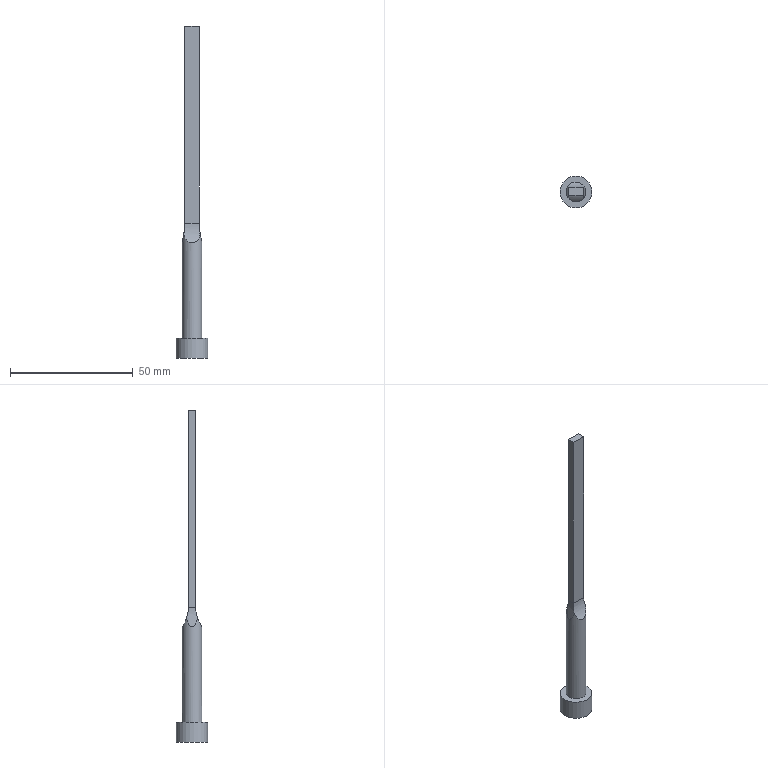Part | STEP file | DDZ8.00_id210_x_t | 1 solid | 13 faces | box 13 x 13 x 135.432 mm | volume 4709 mm3 | plane 7 | cylinder 6 | commonest cylinder face diameters 28.1 x2 65 x2 8 x1 13 x1
STEP:
#1=CARTESIAN_POINT('',(-3.313,-55.759,-85.002));
#2=VERTEX_POINT('',#1);
#3=CARTESIAN_POINT('',(-3.313,-60.241,-85.002));
#4=VERTEX_POINT('',#3);
#5=CARTESIAN_POINT('',(-3.313,-55.759,-85.002));
#6=CARTESIAN_POINT('',(-3.415,-55.909,-85.727));
#7=CARTESIAN_POINT('',(-3.54,-56.104,-86.436));
#8=CARTESIAN_POINT('',(-3.746,-56.586,-87.431));
#9=CARTESIAN_POINT('',(-3.817,-56.776,-87.747));
#10=CARTESIAN_POINT('',(-3.945,-57.286,-88.284));
#11=CARTESIAN_POINT('',(-4.,-57.628,-88.501));
#12=CARTESIAN_POINT('',(-4.,-58.379,-88.499));
#13=CARTESIAN_POINT('',(-3.943,-58.723,-88.276));
#14=CARTESIAN_POINT('',(-3.816,-59.229,-87.74));
#15=CARTESIAN_POINT('',(-3.743,-59.42,-87.42));
#16=CARTESIAN_POINT('',(-3.539,-59.896,-86.433));
#17=CARTESIAN_POINT('',(-3.415,-60.091,-85.726));
#18=CARTESIAN_POINT('',(-3.313,-60.241,-85.002));
#19=B_SPLINE_CURVE_WITH_KNOTS('',3,(#5,#6,#7,#8,#9,#10,#11,#12,#13,#14,#15,#16,#17,#18),.UNSPECIFIED.,.F.,.F.,(4,2,2,2,2,2,4),(0.,0.25,0.375,0.5,0.625,0.75,1.),.UNSPECIFIED.);
#20=EDGE_CURVE('',#2,#4,#19,.T.);
#21=ORIENTED_EDGE('',*,*,#20,.F.);
#22=CARTESIAN_POINT('',(3.313,-55.759,-85.002));
#23=VERTEX_POINT('',#22);
#24=CARTESIAN_POINT('',(3.313,-55.759,-85.002));
#25=CARTESIAN_POINT('',(3.117,-55.468,-85.861));
#26=CARTESIAN_POINT('',(2.822,-55.093,-86.676));
#27=CARTESIAN_POINT('',(1.767,-54.354,-88.002));
#28=CARTESIAN_POINT('',(0.9205,-54.,-88.501));
#29=CARTESIAN_POINT('',(-0.9239,-54.,-88.499));
#30=CARTESIAN_POINT('',(-1.772,-54.357,-87.997));
#31=CARTESIAN_POINT('',(-2.822,-55.094,-86.673));
#32=CARTESIAN_POINT('',(-3.117,-55.469,-85.861));
#33=CARTESIAN_POINT('',(-3.313,-55.759,-85.002));
#34=B_SPLINE_CURVE_WITH_KNOTS('',3,(#24,#25,#26,#27,#28,#29,#30,#31,#32,#33),.UNSPECIFIED.,.F.,.F.,(4,2,2,2,4),(0.,0.25,0.5,0.75,1.),.UNSPECIFIED.);
#35=EDGE_CURVE('',#23,#2,#34,.T.);
#36=ORIENTED_EDGE('',*,*,#35,.F.);
#37=CARTESIAN_POINT('',(3.313,-60.241,-85.002));
#38=VERTEX_POINT('',#37);
#39=CARTESIAN_POINT('',(3.313,-60.241,-85.002));
#40=CARTESIAN_POINT('',(3.415,-60.091,-85.727));
#41=CARTESIAN_POINT('',(3.54,-59.896,-86.436));
#42=CARTESIAN_POINT('',(3.746,-59.414,-87.431));
#43=CARTESIAN_POINT('',(3.817,-59.224,-87.747));
#44=CARTESIAN_POINT('',(3.945,-58.714,-88.284));
#45=CARTESIAN_POINT('',(4.,-58.372,-88.501));
#46=CARTESIAN_POINT('',(4.,-57.621,-88.499));
#47=CARTESIAN_POINT('',(3.943,-57.277,-88.276));
#48=CARTESIAN_POINT('',(3.816,-56.771,-87.74));
#49=CARTESIAN_POINT('',(3.743,-56.58,-87.42));
#50=CARTESIAN_POINT('',(3.539,-56.104,-86.433));
#51=CARTESIAN_POINT('',(3.415,-55.909,-85.726));
#52=CARTESIAN_POINT('',(3.313,-55.759,-85.002));
#53=B_SPLINE_CURVE_WITH_KNOTS('',3,(#39,#40,#41,#42,#43,#44,#45,#46,#47,#48,#49,#50,#51,#52),.UNSPECIFIED.,.F.,.F.,(4,2,2,2,2,2,4),(0.,0.25,0.375,0.5,0.625,0.75,1.),.UNSPECIFIED.);
#54=EDGE_CURVE('',#38,#23,#53,.T.);
#55=ORIENTED_EDGE('',*,*,#54,.F.);
#56=CARTESIAN_POINT('',(-3.313,-60.241,-85.002));
#57=CARTESIAN_POINT('',(-3.117,-60.532,-85.861));
#58=CARTESIAN_POINT('',(-2.822,-60.907,-86.676));
#59=CARTESIAN_POINT('',(-1.767,-61.646,-88.002));
#60=CARTESIAN_POINT('',(-0.9205,-62.,-88.501));
#61=CARTESIAN_POINT('',(0.9239,-62.,-88.499));
#62=CARTESIAN_POINT('',(1.772,-61.643,-87.997));
#63=CARTESIAN_POINT('',(2.822,-60.906,-86.673));
#64=CARTESIAN_POINT('',(3.117,-60.531,-85.861));
#65=CARTESIAN_POINT('',(3.313,-60.241,-85.002));
#66=B_SPLINE_CURVE_WITH_KNOTS('',3,(#56,#57,#58,#59,#60,#61,#62,#63,#64,#65),.UNSPECIFIED.,.F.,.F.,(4,2,2,2,4),(0.,0.25,0.5,0.75,1.),.UNSPECIFIED.);
#67=EDGE_CURVE('',#4,#38,#66,.T.);
#68=ORIENTED_EDGE('',*,*,#67,.F.);
#69=EDGE_LOOP('',(#21,#36,#55,#68));
#70=FACE_BOUND('',#69,.T.);
#71=CARTESIAN_POINT('',(0.,-62.,-127.5));
#72=VERTEX_POINT('',#71);
#73=CARTESIAN_POINT('',(0.,-58.,-127.5));
#74=DIRECTION('',(0.,0.,-1.));
#75=DIRECTION('',(0.,-1.,0.));
#76=AXIS2_PLACEMENT_3D('',#73,#74,#75);
#77=CIRCLE('',#76,4.);
#78=EDGE_CURVE('',#72,#72,#77,.T.);
#79=ORIENTED_EDGE('',*,*,#78,.F.);
#80=EDGE_LOOP('',(#79));
#81=FACE_BOUND('',#80,.T.);
#82=CARTESIAN_POINT('',(0.,-58.,-140.5));
#83=DIRECTION('',(0.,0.,1.));
#84=DIRECTION('',(0.,-1.,0.));
#85=AXIS2_PLACEMENT_3D('',#82,#83,#84);
#86=CYLINDRICAL_SURFACE('',#85,4.);
#87=ADVANCED_FACE('',(#70,#81),#86,.T.);
#88=ORIENTED_EDGE('',*,*,#78,.T.);
#89=EDGE_LOOP('',(#88));
#90=FACE_BOUND('',#89,.T.);
#91=CARTESIAN_POINT('',(0.,-51.5,-127.5));
#92=VERTEX_POINT('',#91);
#93=CARTESIAN_POINT('',(0.,-58.,-127.5));
#94=DIRECTION('',(0.,0.,-1.));
#95=DIRECTION('',(0.,1.,0.));
#96=AXIS2_PLACEMENT_3D('',#93,#94,#95);
#97=CIRCLE('',#96,6.5);
#98=EDGE_CURVE('',#92,#92,#97,.T.);
#99=ORIENTED_EDGE('',*,*,#98,.F.);
#100=EDGE_LOOP('',(#99));
#101=FACE_BOUND('',#100,.T.);
#102=CARTESIAN_POINT('',(0.,-58.,-127.5));
#103=DIRECTION('',(0.,0.,1.));
#104=DIRECTION('',(0.,-1.,0.));
#105=AXIS2_PLACEMENT_3D('',#102,#103,#104);
#106=PLANE('',#105);
#107=ADVANCED_FACE('',(#90,#101),#106,.T.);
#108=ORIENTED_EDGE('',*,*,#98,.T.);
#109=EDGE_LOOP('',(#108));
#110=FACE_BOUND('',#109,.T.);
#111=CARTESIAN_POINT('',(0.,-64.5,-135.5));
#112=VERTEX_POINT('',#111);
#113=CARTESIAN_POINT('',(0.,-58.,-135.5));
#114=DIRECTION('',(0.,0.,1.));
#115=DIRECTION('',(0.,-1.,0.));
#116=AXIS2_PLACEMENT_3D('',#113,#114,#115);
#117=CIRCLE('',#116,6.5);
#118=EDGE_CURVE('',#112,#112,#117,.T.);
#119=ORIENTED_EDGE('',*,*,#118,.T.);
#120=EDGE_LOOP('',(#119));
#121=FACE_BOUND('',#120,.T.);
#122=CARTESIAN_POINT('',(0.,-58.,-135.5));
#123=DIRECTION('',(0.,0.,1.));
#124=DIRECTION('',(0.,-1.,0.));
#125=AXIS2_PLACEMENT_3D('',#122,#123,#124);
#126=CYLINDRICAL_SURFACE('',#125,6.5);
#127=ADVANCED_FACE('',(#110,#121),#126,.T.);
#128=ORIENTED_EDGE('',*,*,#118,.F.);
#129=EDGE_LOOP('',(#128));
#130=FACE_OUTER_BOUND('',#129,.T.);
#131=CARTESIAN_POINT('',(0.,-58.,-135.5));
#132=DIRECTION('',(0.,0.,-1.));
#133=DIRECTION('',(0.,1.,0.));
#134=AXIS2_PLACEMENT_3D('',#131,#132,#133);
#135=PLANE('',#134);
#136=ADVANCED_FACE('',(#130),#135,.T.);
#137=CARTESIAN_POINT('',(-3.,-59.5,-0.06829));
#138=VERTEX_POINT('',#137);
#139=CARTESIAN_POINT('',(-3.,-56.5,-0.06829));
#140=VERTEX_POINT('',#139);
#141=CARTESIAN_POINT('',(-3.,-58.,-0.06829));
#142=DIRECTION('',(0.,1.,0.));
#143=VECTOR('',#142,1.);
#144=LINE('',#141,#143);
#145=EDGE_CURVE('',#138,#140,#144,.T.);
#146=ORIENTED_EDGE('',*,*,#145,.F.);
#147=CARTESIAN_POINT('',(3.,-59.5,-0.173));
#148=VERTEX_POINT('',#147);
#149=CARTESIAN_POINT('',(-1.04,-59.5,-0.1025));
#150=DIRECTION('',(-0.9998,0.,0.01745));
#151=VECTOR('',#150,1.);
#152=LINE('',#149,#151);
#153=EDGE_CURVE('',#148,#138,#152,.T.);
#154=ORIENTED_EDGE('',*,*,#153,.F.);
#155=CARTESIAN_POINT('',(3.,-56.5,-0.173));
#156=VERTEX_POINT('',#155);
#157=CARTESIAN_POINT('',(3.,-58.,-0.173));
#158=DIRECTION('',(0.,-1.,0.));
#159=VECTOR('',#158,1.);
#160=LINE('',#157,#159);
#161=EDGE_CURVE('',#156,#148,#160,.T.);
#162=ORIENTED_EDGE('',*,*,#161,.F.);
#163=CARTESIAN_POINT('',(-1.04,-56.5,-0.1025));
#164=DIRECTION('',(0.9998,0.,-0.01745));
#165=VECTOR('',#164,1.);
#166=LINE('',#163,#165);
#167=EDGE_CURVE('',#140,#156,#166,.T.);
#168=ORIENTED_EDGE('',*,*,#167,.F.);
#169=EDGE_LOOP('',(#146,#154,#162,#168));
#170=FACE_OUTER_BOUND('',#169,.T.);
#171=CARTESIAN_POINT('',(0.01744,-55.5,-0.121));
#172=DIRECTION('',(-0.01745,0.,-0.9998));
#173=DIRECTION('',(0.,1.,0.));
#174=AXIS2_PLACEMENT_3D('',#171,#172,#173);
#175=PLANE('',#174);
#176=ADVANCED_FACE('',(#170),#175,.F.);
#177=CARTESIAN_POINT('',(-3.,-59.5,-80.5));
#178=VERTEX_POINT('',#177);
#179=CARTESIAN_POINT('',(-3.,-59.5,59.5));
#180=DIRECTION('',(0.,0.,1.));
#181=VECTOR('',#180,1.);
#182=LINE('',#179,#181);
#183=EDGE_CURVE('',#178,#138,#182,.T.);
#184=ORIENTED_EDGE('',*,*,#183,.T.);
#185=ORIENTED_EDGE('',*,*,#145,.T.);
#186=CARTESIAN_POINT('',(-3.,-56.5,-80.5));
#187=VERTEX_POINT('',#186);
#188=CARTESIAN_POINT('',(-3.,-56.5,59.5));
#189=DIRECTION('',(0.,0.,1.));
#190=VECTOR('',#189,1.);
#191=LINE('',#188,#190);
#192=EDGE_CURVE('',#187,#140,#191,.T.);
#193=ORIENTED_EDGE('',*,*,#192,.F.);
#194=CARTESIAN_POINT('',(-3.,-58.,-80.5));
#195=DIRECTION('',(0.,-1.,0.));
#196=VECTOR('',#195,1.);
#197=LINE('',#194,#196);
#198=EDGE_CURVE('',#187,#178,#197,.T.);
#199=ORIENTED_EDGE('',*,*,#198,.T.);
#200=EDGE_LOOP('',(#184,#185,#193,#199));
#201=FACE_OUTER_BOUND('',#200,.T.);
#202=CARTESIAN_POINT('',(-3.,-58.,59.5));
#203=DIRECTION('',(-1.,0.,0.));
#204=DIRECTION('',(0.,0.,-1.));
#205=AXIS2_PLACEMENT_3D('',#202,#203,#204);
#206=PLANE('',#205);
#207=ADVANCED_FACE('',(#201),#206,.T.);
#208=ORIENTED_EDGE('',*,*,#192,.T.);
#209=ORIENTED_EDGE('',*,*,#167,.T.);
#210=CARTESIAN_POINT('',(3.,-56.5,-80.5));
#211=VERTEX_POINT('',#210);
#212=CARTESIAN_POINT('',(3.,-56.5,59.5));
#213=DIRECTION('',(0.,0.,1.));
#214=VECTOR('',#213,1.);
#215=LINE('',#212,#214);
#216=EDGE_CURVE('',#211,#156,#215,.T.);
#217=ORIENTED_EDGE('',*,*,#216,.F.);
#218=CARTESIAN_POINT('',(0.,-56.5,-80.5));
#219=DIRECTION('',(-1.,0.,0.));
#220=VECTOR('',#219,1.);
#221=LINE('',#218,#220);
#222=EDGE_CURVE('',#211,#187,#221,.T.);
#223=ORIENTED_EDGE('',*,*,#222,.T.);
#224=EDGE_LOOP('',(#208,#209,#217,#223));
#225=FACE_OUTER_BOUND('',#224,.T.);
#226=CARTESIAN_POINT('',(0.,-56.5,59.5));
#227=DIRECTION('',(0.,1.,0.));
#228=DIRECTION('',(0.,0.,1.));
#229=AXIS2_PLACEMENT_3D('',#226,#227,#228);
#230=PLANE('',#229);
#231=ADVANCED_FACE('',(#225),#230,.T.);
#232=ORIENTED_EDGE('',*,*,#216,.T.);
#233=ORIENTED_EDGE('',*,*,#161,.T.);
#234=CARTESIAN_POINT('',(3.,-59.5,-80.5));
#235=VERTEX_POINT('',#234);
#236=CARTESIAN_POINT('',(3.,-59.5,59.5));
#237=DIRECTION('',(0.,0.,1.));
#238=VECTOR('',#237,1.);
#239=LINE('',#236,#238);
#240=EDGE_CURVE('',#235,#148,#239,.T.);
#241=ORIENTED_EDGE('',*,*,#240,.F.);
#242=CARTESIAN_POINT('',(3.,-58.,-80.5));
#243=DIRECTION('',(0.,1.,0.));
#244=VECTOR('',#243,1.);
#245=LINE('',#242,#244);
#246=EDGE_CURVE('',#235,#211,#245,.T.);
#247=ORIENTED_EDGE('',*,*,#246,.T.);
#248=EDGE_LOOP('',(#232,#233,#241,#247));
#249=FACE_OUTER_BOUND('',#248,.T.);
#250=CARTESIAN_POINT('',(3.,-58.,59.5));
#251=DIRECTION('',(1.,0.,0.));
#252=DIRECTION('',(0.,0.,1.));
#253=AXIS2_PLACEMENT_3D('',#250,#251,#252);
#254=PLANE('',#253);
#255=ADVANCED_FACE('',(#249),#254,.T.);
#256=CARTESIAN_POINT('',(0.,-59.5,-80.5));
#257=DIRECTION('',(1.,0.,0.));
#258=VECTOR('',#257,1.);
#259=LINE('',#256,#258);
#260=EDGE_CURVE('',#178,#235,#259,.T.);
#261=ORIENTED_EDGE('',*,*,#260,.T.);
#262=ORIENTED_EDGE('',*,*,#240,.T.);
#263=ORIENTED_EDGE('',*,*,#153,.T.);
#264=ORIENTED_EDGE('',*,*,#183,.F.);
#265=EDGE_LOOP('',(#261,#262,#263,#264));
#266=FACE_OUTER_BOUND('',#265,.T.);
#267=CARTESIAN_POINT('',(0.,-59.5,59.5));
#268=DIRECTION('',(0.,-1.,0.));
#269=DIRECTION('',(0.,0.,-1.));
#270=AXIS2_PLACEMENT_3D('',#267,#268,#269);
#271=PLANE('',#270);
#272=ADVANCED_FACE('',(#266),#271,.T.);
#273=ORIENTED_EDGE('',*,*,#260,.F.);
#274=CARTESIAN_POINT('',(-3.,-59.5,-80.5));
#275=CARTESIAN_POINT('',(-3.,-59.5,-82.048));
#276=CARTESIAN_POINT('',(-3.11,-59.75,-83.55));
#277=CARTESIAN_POINT('',(-3.313,-60.241,-85.002));
#278=B_SPLINE_CURVE_WITH_KNOTS('',3,(#274,#275,#276,#277),.UNSPECIFIED.,.F.,.F.,(4,4),(0.,1.),.UNSPECIFIED.);
#279=EDGE_CURVE('',#178,#4,#278,.T.);
#280=ORIENTED_EDGE('',*,*,#279,.T.);
#281=ORIENTED_EDGE('',*,*,#67,.T.);
#282=CARTESIAN_POINT('',(3.313,-60.241,-85.002));
#283=CARTESIAN_POINT('',(3.114,-59.758,-83.575));
#284=CARTESIAN_POINT('',(3.,-59.5,-82.041));
#285=CARTESIAN_POINT('',(3.,-59.5,-80.5));
#286=B_SPLINE_CURVE_WITH_KNOTS('',3,(#282,#283,#284,#285),.UNSPECIFIED.,.F.,.F.,(4,4),(0.,1.),.UNSPECIFIED.);
#287=EDGE_CURVE('',#38,#235,#286,.T.);
#288=ORIENTED_EDGE('',*,*,#287,.T.);
#289=EDGE_LOOP('',(#273,#280,#281,#288));
#290=FACE_OUTER_BOUND('',#289,.T.);
#291=CARTESIAN_POINT('',(20.,-73.55,-80.5));
#292=DIRECTION('',(-1.,0.,0.));
#293=DIRECTION('',(0.,0.,-1.));
#294=AXIS2_PLACEMENT_3D('',#291,#292,#293);
#295=CYLINDRICAL_SURFACE('',#294,14.05);
#296=ADVANCED_FACE('',(#290),#295,.F.);
#297=ORIENTED_EDGE('',*,*,#35,.T.);
#298=CARTESIAN_POINT('',(-3.313,-55.759,-85.002));
#299=CARTESIAN_POINT('',(-3.114,-56.242,-83.575));
#300=CARTESIAN_POINT('',(-3.,-56.5,-82.041));
#301=CARTESIAN_POINT('',(-3.,-56.5,-80.5));
#302=B_SPLINE_CURVE_WITH_KNOTS('',3,(#298,#299,#300,#301),.UNSPECIFIED.,.F.,.F.,(4,4),(0.,1.),.UNSPECIFIED.);
#303=EDGE_CURVE('',#2,#187,#302,.T.);
#304=ORIENTED_EDGE('',*,*,#303,.T.);
#305=ORIENTED_EDGE('',*,*,#222,.F.);
#306=CARTESIAN_POINT('',(3.,-56.5,-80.5));
#307=CARTESIAN_POINT('',(3.,-56.5,-82.048));
#308=CARTESIAN_POINT('',(3.11,-56.25,-83.55));
#309=CARTESIAN_POINT('',(3.313,-55.759,-85.002));
#310=B_SPLINE_CURVE_WITH_KNOTS('',3,(#306,#307,#308,#309),.UNSPECIFIED.,.F.,.F.,(4,4),(0.,1.),.UNSPECIFIED.);
#311=EDGE_CURVE('',#211,#23,#310,.T.);
#312=ORIENTED_EDGE('',*,*,#311,.T.);
#313=EDGE_LOOP('',(#297,#304,#305,#312));
#314=FACE_OUTER_BOUND('',#313,.T.);
#315=CARTESIAN_POINT('',(20.,-42.45,-80.5));
#316=DIRECTION('',(-1.,0.,0.));
#317=DIRECTION('',(0.,0.,-1.));
#318=AXIS2_PLACEMENT_3D('',#315,#316,#317);
#319=CYLINDRICAL_SURFACE('',#318,14.05);
#320=ADVANCED_FACE('',(#314),#319,.F.);
#321=ORIENTED_EDGE('',*,*,#54,.T.);
#322=ORIENTED_EDGE('',*,*,#311,.F.);
#323=ORIENTED_EDGE('',*,*,#246,.F.);
#324=ORIENTED_EDGE('',*,*,#287,.F.);
#325=EDGE_LOOP('',(#321,#322,#323,#324));
#326=FACE_OUTER_BOUND('',#325,.T.);
#327=CARTESIAN_POINT('',(35.5,-78.,-80.5));
#328=DIRECTION('',(0.,1.,0.));
#329=DIRECTION('',(0.,0.,1.));
#330=AXIS2_PLACEMENT_3D('',#327,#328,#329);
#331=CYLINDRICAL_SURFACE('',#330,32.5);
#332=ADVANCED_FACE('',(#326),#331,.F.);
#333=ORIENTED_EDGE('',*,*,#198,.F.);
#334=ORIENTED_EDGE('',*,*,#303,.F.);
#335=ORIENTED_EDGE('',*,*,#20,.T.);
#336=ORIENTED_EDGE('',*,*,#279,.F.);
#337=EDGE_LOOP('',(#333,#334,#335,#336));
#338=FACE_OUTER_BOUND('',#337,.T.);
#339=CARTESIAN_POINT('',(-35.5,-78.,-80.5));
#340=DIRECTION('',(0.,1.,0.));
#341=DIRECTION('',(0.,0.,1.));
#342=AXIS2_PLACEMENT_3D('',#339,#340,#341);
#343=CYLINDRICAL_SURFACE('',#342,32.5);
#344=ADVANCED_FACE('',(#338),#343,.F.);
#345=CLOSED_SHELL('',(#87,#107,#127,#136,#176,#207,#231,#255,#272,#296,#320,#332,#344));
#346=MANIFOLD_SOLID_BREP('',#345);
#347=(LENGTH_UNIT()NAMED_UNIT(*)SI_UNIT(.MILLI.,.METRE.));
#348=UNCERTAINTY_MEASURE_WITH_UNIT(LENGTH_MEASURE(0.0508),#347,'','');
#349=(NAMED_UNIT(*)PLANE_ANGLE_UNIT()SI_UNIT($,.RADIAN.));
#350=PLANE_ANGLE_MEASURE_WITH_UNIT(PLANE_ANGLE_MEASURE(0.01745),#349);
#351=DIMENSIONAL_EXPONENTS(0.,0.,0.,0.,0.,0.,0.);
#352=(CONVERSION_BASED_UNIT('DEGREE',#350)NAMED_UNIT(#351)PLANE_ANGLE_UNIT());
#353=(NAMED_UNIT(*)SI_UNIT($,.STERADIAN.)SOLID_ANGLE_UNIT());
#354=(GEOMETRIC_REPRESENTATION_CONTEXT(3)GLOBAL_UNCERTAINTY_ASSIGNED_CONTEXT((#348))GLOBAL_UNIT_ASSIGNED_CONTEXT((#347,#352,#353))REPRESENTATION_CONTEXT('',''));
#355=ADVANCED_BREP_SHAPE_REPRESENTATION('',(#346),#354);